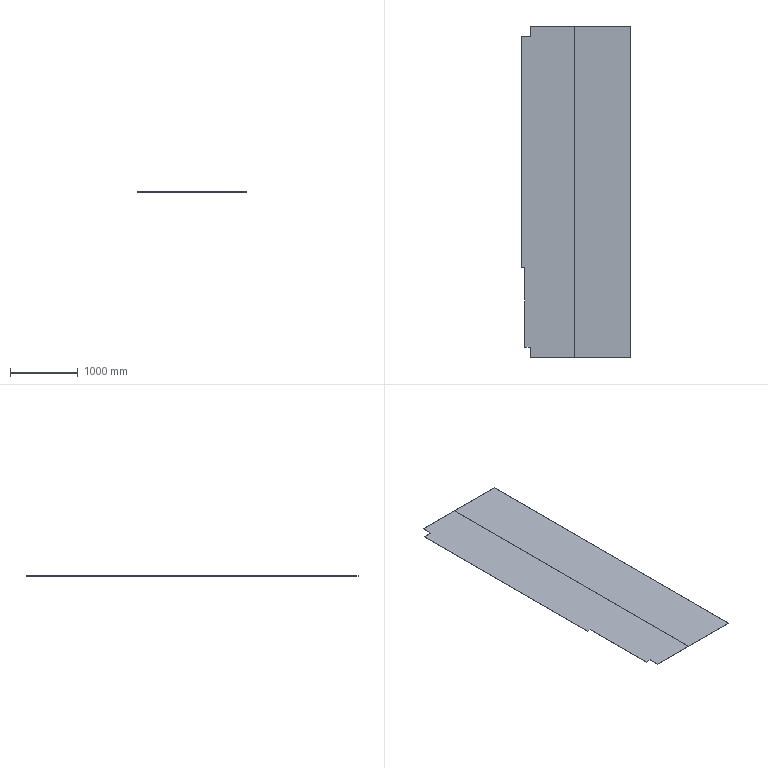Part | STEP file | 休息台花纹Plate 2 | 2 solids | 18 faces | box 1620 x 4900 x 3 mm | volume 23500005 mm3 | plane 18
STEP:
#1=CARTESIAN_POINT('',(0.,0.,0.));
#2=DIRECTION('',(0.,0.,1.));
#3=DIRECTION('',(1.,0.,0.));
#4=AXIS2_PLACEMENT_3D('',#1,#2,#3);
#5=CARTESIAN_POINT('',(-565.,50.,3.));
#6=VERTEX_POINT('',#5);
#7=CARTESIAN_POINT('',(-565.,50.,0.));
#8=VERTEX_POINT('',#7);
#9=CARTESIAN_POINT('',(-565.,50.,3.));
#10=DIRECTION('',(0.,0.,-1.));
#11=VECTOR('',#10,1.);
#12=LINE('',#9,#11);
#13=CARTESIAN_POINT('',(-565.,50.,-0.01));
#14=DIRECTION('',(-1.,0.,0.));
#15=DIRECTION('',(0.,-1.,0.));
#16=AXIS2_PLACEMENT_3D('',#13,#14,#15);
#17=PLANE('',#16);
#18=CARTESIAN_POINT('',(0.,3.01));
#19=DIRECTION('',(0.,-1.));
#20=VECTOR('',#19,1.);
#21=LINE('',#18,#20);
#22=(GEOMETRIC_REPRESENTATION_CONTEXT(2)PARAMETRIC_REPRESENTATION_CONTEXT()REPRESENTATION_CONTEXT('',''));
#23=DEFINITIONAL_REPRESENTATION('',(#21),#22);
#24=PCURVE('',#17,#23);
#25=CARTESIAN_POINT('',(270.,50.,3.));
#26=DIRECTION('',(0.,-1.,0.));
#27=DIRECTION('',(0.,0.,-1.));
#28=AXIS2_PLACEMENT_3D('',#25,#26,#27);
#29=PLANE('',#28);
#30=CARTESIAN_POINT('',(0.,-835.));
#31=DIRECTION('',(1.,0.));
#32=VECTOR('',#31,1.);
#33=LINE('',#30,#32);
#34=(GEOMETRIC_REPRESENTATION_CONTEXT(2)PARAMETRIC_REPRESENTATION_CONTEXT()REPRESENTATION_CONTEXT('',''));
#35=DEFINITIONAL_REPRESENTATION('',(#33),#34);
#36=PCURVE('',#29,#35);
#37=SURFACE_CURVE('',#12,(#24,#36),.PCURVE_S1.);
#38=EDGE_CURVE('',#6,#8,#37,.T.);
#39=ORIENTED_EDGE('',*,*,#38,.F.);
#40=CARTESIAN_POINT('',(-565.,-4850.,3.));
#41=VERTEX_POINT('',#40);
#42=CARTESIAN_POINT('',(-565.,0.,3.));
#43=DIRECTION('',(0.,-1.,0.));
#44=VECTOR('',#43,1.);
#45=LINE('',#42,#44);
#46=CARTESIAN_POINT('',(50.,3.01));
#47=DIRECTION('',(1.,0.));
#48=VECTOR('',#47,1.);
#49=LINE('',#46,#48);
#50=(GEOMETRIC_REPRESENTATION_CONTEXT(2)PARAMETRIC_REPRESENTATION_CONTEXT()REPRESENTATION_CONTEXT('',''));
#51=DEFINITIONAL_REPRESENTATION('',(#49),#50);
#52=PCURVE('',#17,#51);
#53=CARTESIAN_POINT('',(0.,0.,3.));
#54=DIRECTION('',(0.,0.,1.));
#55=DIRECTION('',(1.,0.,0.));
#56=AXIS2_PLACEMENT_3D('',#53,#54,#55);
#57=PLANE('',#56);
#58=CARTESIAN_POINT('',(-565.,0.));
#59=DIRECTION('',(0.,-1.));
#60=VECTOR('',#59,1.);
#61=LINE('',#58,#60);
#62=(GEOMETRIC_REPRESENTATION_CONTEXT(2)PARAMETRIC_REPRESENTATION_CONTEXT()REPRESENTATION_CONTEXT('',''));
#63=DEFINITIONAL_REPRESENTATION('',(#61),#62);
#64=PCURVE('',#57,#63);
#65=SURFACE_CURVE('',#45,(#52,#64),.PCURVE_S1.);
#66=EDGE_CURVE('',#6,#41,#65,.T.);
#67=ORIENTED_EDGE('',*,*,#66,.T.);
#68=CARTESIAN_POINT('',(-565.,-4850.,0.));
#69=VERTEX_POINT('',#68);
#70=CARTESIAN_POINT('',(-565.,-4850.,3.));
#71=DIRECTION('',(0.,0.,1.));
#72=VECTOR('',#71,1.);
#73=LINE('',#70,#72);
#74=CARTESIAN_POINT('',(4900.,3.01));
#75=DIRECTION('',(0.,1.));
#76=VECTOR('',#75,1.);
#77=LINE('',#74,#76);
#78=(GEOMETRIC_REPRESENTATION_CONTEXT(2)PARAMETRIC_REPRESENTATION_CONTEXT()REPRESENTATION_CONTEXT('',''));
#79=DEFINITIONAL_REPRESENTATION('',(#77),#78);
#80=PCURVE('',#17,#79);
#81=CARTESIAN_POINT('',(-1215.,-4850.,3.));
#82=DIRECTION('',(0.,1.,0.));
#83=DIRECTION('',(0.,0.,1.));
#84=AXIS2_PLACEMENT_3D('',#81,#82,#83);
#85=PLANE('',#84);
#86=CARTESIAN_POINT('',(0.,650.));
#87=DIRECTION('',(1.,0.));
#88=VECTOR('',#87,1.);
#89=LINE('',#86,#88);
#90=(GEOMETRIC_REPRESENTATION_CONTEXT(2)PARAMETRIC_REPRESENTATION_CONTEXT()REPRESENTATION_CONTEXT('',''));
#91=DEFINITIONAL_REPRESENTATION('',(#89),#90);
#92=PCURVE('',#85,#91);
#93=SURFACE_CURVE('',#73,(#80,#92),.PCURVE_S1.);
#94=EDGE_CURVE('',#69,#41,#93,.T.);
#95=ORIENTED_EDGE('',*,*,#94,.F.);
#96=CARTESIAN_POINT('',(-565.,0.,0.));
#97=DIRECTION('',(0.,-1.,0.));
#98=VECTOR('',#97,1.);
#99=LINE('',#96,#98);
#100=CARTESIAN_POINT('',(50.,0.01));
#101=DIRECTION('',(1.,0.));
#102=VECTOR('',#101,1.);
#103=LINE('',#100,#102);
#104=(GEOMETRIC_REPRESENTATION_CONTEXT(2)PARAMETRIC_REPRESENTATION_CONTEXT()REPRESENTATION_CONTEXT('',''));
#105=DEFINITIONAL_REPRESENTATION('',(#103),#104);
#106=PCURVE('',#17,#105);
#107=CARTESIAN_POINT('',(0.,0.,0.));
#108=DIRECTION('',(0.,0.,1.));
#109=DIRECTION('',(1.,0.,0.));
#110=AXIS2_PLACEMENT_3D('',#107,#108,#109);
#111=PLANE('',#110);
#112=CARTESIAN_POINT('',(-565.,0.));
#113=DIRECTION('',(0.,-1.));
#114=VECTOR('',#113,1.);
#115=LINE('',#112,#114);
#116=(GEOMETRIC_REPRESENTATION_CONTEXT(2)PARAMETRIC_REPRESENTATION_CONTEXT()REPRESENTATION_CONTEXT('',''));
#117=DEFINITIONAL_REPRESENTATION('',(#115),#116);
#118=PCURVE('',#111,#117);
#119=SURFACE_CURVE('',#99,(#106,#118),.PCURVE_S1.);
#120=EDGE_CURVE('',#8,#69,#119,.T.);
#121=ORIENTED_EDGE('',*,*,#120,.F.);
#122=EDGE_LOOP('',(#39,#67,#95,#121));
#123=FACE_BOUND('',#122,.T.);
#124=ADVANCED_FACE('',(#123),#17,.F.);
#125=ORIENTED_EDGE('',*,*,#66,.F.);
#126=CARTESIAN_POINT('',(-1215.,50.,3.));
#127=VERTEX_POINT('',#126);
#128=CARTESIAN_POINT('',(270.,50.,3.));
#129=DIRECTION('',(-1.,0.,0.));
#130=VECTOR('',#129,1.);
#131=LINE('',#128,#130);
#132=CARTESIAN_POINT('',(270.,50.));
#133=DIRECTION('',(-1.,0.));
#134=VECTOR('',#133,1.);
#135=LINE('',#132,#134);
#136=(GEOMETRIC_REPRESENTATION_CONTEXT(2)PARAMETRIC_REPRESENTATION_CONTEXT()REPRESENTATION_CONTEXT('',''));
#137=DEFINITIONAL_REPRESENTATION('',(#135),#136);
#138=PCURVE('',#57,#137);
#139=CARTESIAN_POINT('',(0.,0.));
#140=DIRECTION('',(0.,-1.));
#141=VECTOR('',#140,1.);
#142=LINE('',#139,#141);
#143=(GEOMETRIC_REPRESENTATION_CONTEXT(2)PARAMETRIC_REPRESENTATION_CONTEXT()REPRESENTATION_CONTEXT('',''));
#144=DEFINITIONAL_REPRESENTATION('',(#142),#143);
#145=PCURVE('',#29,#144);
#146=SURFACE_CURVE('',#131,(#138,#145),.PCURVE_S1.);
#147=EDGE_CURVE('',#6,#127,#146,.T.);
#148=ORIENTED_EDGE('',*,*,#147,.T.);
#149=CARTESIAN_POINT('',(-1215.,-107.,3.));
#150=VERTEX_POINT('',#149);
#151=CARTESIAN_POINT('',(-1215.,50.,3.));
#152=DIRECTION('',(0.,-1.,0.));
#153=VECTOR('',#152,1.);
#154=LINE('',#151,#153);
#155=CARTESIAN_POINT('',(-1215.,50.));
#156=DIRECTION('',(0.,-1.));
#157=VECTOR('',#156,1.);
#158=LINE('',#155,#157);
#159=(GEOMETRIC_REPRESENTATION_CONTEXT(2)PARAMETRIC_REPRESENTATION_CONTEXT()REPRESENTATION_CONTEXT('',''));
#160=DEFINITIONAL_REPRESENTATION('',(#158),#159);
#161=PCURVE('',#57,#160);
#162=CARTESIAN_POINT('',(-1215.,50.,3.));
#163=DIRECTION('',(1.,0.,0.));
#164=DIRECTION('',(0.,0.,-1.));
#165=AXIS2_PLACEMENT_3D('',#162,#163,#164);
#166=PLANE('',#165);
#167=CARTESIAN_POINT('',(0.,0.));
#168=DIRECTION('',(0.,-1.));
#169=VECTOR('',#168,1.);
#170=LINE('',#167,#169);
#171=(GEOMETRIC_REPRESENTATION_CONTEXT(2)PARAMETRIC_REPRESENTATION_CONTEXT()REPRESENTATION_CONTEXT('',''));
#172=DEFINITIONAL_REPRESENTATION('',(#170),#171);
#173=PCURVE('',#166,#172);
#174=SURFACE_CURVE('',#154,(#161,#173),.PCURVE_S1.);
#175=EDGE_CURVE('',#127,#150,#174,.T.);
#176=ORIENTED_EDGE('',*,*,#175,.T.);
#177=CARTESIAN_POINT('',(-1350.,-107.,3.));
#178=VERTEX_POINT('',#177);
#179=CARTESIAN_POINT('',(-1215.,-107.,3.));
#180=DIRECTION('',(-1.,0.,0.));
#181=VECTOR('',#180,1.);
#182=LINE('',#179,#181);
#183=CARTESIAN_POINT('',(-1215.,-107.));
#184=DIRECTION('',(-1.,0.));
#185=VECTOR('',#184,1.);
#186=LINE('',#183,#185);
#187=(GEOMETRIC_REPRESENTATION_CONTEXT(2)PARAMETRIC_REPRESENTATION_CONTEXT()REPRESENTATION_CONTEXT('',''));
#188=DEFINITIONAL_REPRESENTATION('',(#186),#187);
#189=PCURVE('',#57,#188);
#190=CARTESIAN_POINT('',(-1215.,-107.,3.));
#191=DIRECTION('',(0.,-1.,0.));
#192=DIRECTION('',(0.,0.,-1.));
#193=AXIS2_PLACEMENT_3D('',#190,#191,#192);
#194=PLANE('',#193);
#195=CARTESIAN_POINT('',(0.,0.));
#196=DIRECTION('',(0.,-1.));
#197=VECTOR('',#196,1.);
#198=LINE('',#195,#197);
#199=(GEOMETRIC_REPRESENTATION_CONTEXT(2)PARAMETRIC_REPRESENTATION_CONTEXT()REPRESENTATION_CONTEXT('',''));
#200=DEFINITIONAL_REPRESENTATION('',(#198),#199);
#201=PCURVE('',#194,#200);
#202=SURFACE_CURVE('',#182,(#189,#201),.PCURVE_S1.);
#203=EDGE_CURVE('',#150,#178,#202,.T.);
#204=ORIENTED_EDGE('',*,*,#203,.T.);
#205=CARTESIAN_POINT('',(-1350.,-3518.,3.));
#206=VERTEX_POINT('',#205);
#207=CARTESIAN_POINT('',(-1350.,-107.,3.));
#208=DIRECTION('',(0.,-1.,0.));
#209=VECTOR('',#208,1.);
#210=LINE('',#207,#209);
#211=CARTESIAN_POINT('',(-1350.,-107.));
#212=DIRECTION('',(0.,-1.));
#213=VECTOR('',#212,1.);
#214=LINE('',#211,#213);
#215=(GEOMETRIC_REPRESENTATION_CONTEXT(2)PARAMETRIC_REPRESENTATION_CONTEXT()REPRESENTATION_CONTEXT('',''));
#216=DEFINITIONAL_REPRESENTATION('',(#214),#215);
#217=PCURVE('',#57,#216);
#218=CARTESIAN_POINT('',(-1350.,-107.,3.));
#219=DIRECTION('',(1.,0.,0.));
#220=DIRECTION('',(0.,1.,0.));
#221=AXIS2_PLACEMENT_3D('',#218,#219,#220);
#222=PLANE('',#221);
#223=CARTESIAN_POINT('',(0.,0.));
#224=DIRECTION('',(-1.,0.));
#225=VECTOR('',#224,1.);
#226=LINE('',#223,#225);
#227=(GEOMETRIC_REPRESENTATION_CONTEXT(2)PARAMETRIC_REPRESENTATION_CONTEXT()REPRESENTATION_CONTEXT('',''));
#228=DEFINITIONAL_REPRESENTATION('',(#226),#227);
#229=PCURVE('',#222,#228);
#230=SURFACE_CURVE('',#210,(#217,#229),.PCURVE_S1.);
#231=EDGE_CURVE('',#178,#206,#230,.T.);
#232=ORIENTED_EDGE('',*,*,#231,.T.);
#233=CARTESIAN_POINT('',(-1297.,-3518.,3.));
#234=VERTEX_POINT('',#233);
#235=CARTESIAN_POINT('',(-1350.,-3518.,3.));
#236=DIRECTION('',(1.,0.,0.));
#237=VECTOR('',#236,1.);
#238=LINE('',#235,#237);
#239=CARTESIAN_POINT('',(-1350.,-3518.));
#240=DIRECTION('',(1.,0.));
#241=VECTOR('',#240,1.);
#242=LINE('',#239,#241);
#243=(GEOMETRIC_REPRESENTATION_CONTEXT(2)PARAMETRIC_REPRESENTATION_CONTEXT()REPRESENTATION_CONTEXT('',''));
#244=DEFINITIONAL_REPRESENTATION('',(#242),#243);
#245=PCURVE('',#57,#244);
#246=CARTESIAN_POINT('',(-1350.,-3518.,3.));
#247=DIRECTION('',(0.,1.,0.));
#248=DIRECTION('',(0.,0.,1.));
#249=AXIS2_PLACEMENT_3D('',#246,#247,#248);
#250=PLANE('',#249);
#251=CARTESIAN_POINT('',(0.,0.));
#252=DIRECTION('',(0.,1.));
#253=VECTOR('',#252,1.);
#254=LINE('',#251,#253);
#255=(GEOMETRIC_REPRESENTATION_CONTEXT(2)PARAMETRIC_REPRESENTATION_CONTEXT()REPRESENTATION_CONTEXT('',''));
#256=DEFINITIONAL_REPRESENTATION('',(#254),#255);
#257=PCURVE('',#250,#256);
#258=SURFACE_CURVE('',#238,(#245,#257),.PCURVE_S1.);
#259=EDGE_CURVE('',#206,#234,#258,.T.);
#260=ORIENTED_EDGE('',*,*,#259,.T.);
#261=CARTESIAN_POINT('',(-1297.,-4693.,3.));
#262=VERTEX_POINT('',#261);
#263=CARTESIAN_POINT('',(-1297.,-3518.,3.));
#264=DIRECTION('',(0.,-1.,0.));
#265=VECTOR('',#264,1.);
#266=LINE('',#263,#265);
#267=CARTESIAN_POINT('',(-1297.,-3518.));
#268=DIRECTION('',(0.,-1.));
#269=VECTOR('',#268,1.);
#270=LINE('',#267,#269);
#271=(GEOMETRIC_REPRESENTATION_CONTEXT(2)PARAMETRIC_REPRESENTATION_CONTEXT()REPRESENTATION_CONTEXT('',''));
#272=DEFINITIONAL_REPRESENTATION('',(#270),#271);
#273=PCURVE('',#57,#272);
#274=CARTESIAN_POINT('',(-1297.,-3518.,3.));
#275=DIRECTION('',(1.,0.,0.));
#276=DIRECTION('',(0.,1.,0.));
#277=AXIS2_PLACEMENT_3D('',#274,#275,#276);
#278=PLANE('',#277);
#279=CARTESIAN_POINT('',(0.,0.));
#280=DIRECTION('',(-1.,0.));
#281=VECTOR('',#280,1.);
#282=LINE('',#279,#281);
#283=(GEOMETRIC_REPRESENTATION_CONTEXT(2)PARAMETRIC_REPRESENTATION_CONTEXT()REPRESENTATION_CONTEXT('',''));
#284=DEFINITIONAL_REPRESENTATION('',(#282),#283);
#285=PCURVE('',#278,#284);
#286=SURFACE_CURVE('',#266,(#273,#285),.PCURVE_S1.);
#287=EDGE_CURVE('',#234,#262,#286,.T.);
#288=ORIENTED_EDGE('',*,*,#287,.T.);
#289=CARTESIAN_POINT('',(-1215.,-4693.,3.));
#290=VERTEX_POINT('',#289);
#291=CARTESIAN_POINT('',(-1297.,-4693.,3.));
#292=DIRECTION('',(1.,0.,0.));
#293=VECTOR('',#292,1.);
#294=LINE('',#291,#293);
#295=CARTESIAN_POINT('',(-1297.,-4693.));
#296=DIRECTION('',(1.,0.));
#297=VECTOR('',#296,1.);
#298=LINE('',#295,#297);
#299=(GEOMETRIC_REPRESENTATION_CONTEXT(2)PARAMETRIC_REPRESENTATION_CONTEXT()REPRESENTATION_CONTEXT('',''));
#300=DEFINITIONAL_REPRESENTATION('',(#298),#299);
#301=PCURVE('',#57,#300);
#302=CARTESIAN_POINT('',(-1297.,-4693.,3.));
#303=DIRECTION('',(0.,1.,0.));
#304=DIRECTION('',(0.,0.,1.));
#305=AXIS2_PLACEMENT_3D('',#302,#303,#304);
#306=PLANE('',#305);
#307=CARTESIAN_POINT('',(0.,0.));
#308=DIRECTION('',(0.,1.));
#309=VECTOR('',#308,1.);
#310=LINE('',#307,#309);
#311=(GEOMETRIC_REPRESENTATION_CONTEXT(2)PARAMETRIC_REPRESENTATION_CONTEXT()REPRESENTATION_CONTEXT('',''));
#312=DEFINITIONAL_REPRESENTATION('',(#310),#311);
#313=PCURVE('',#306,#312);
#314=SURFACE_CURVE('',#294,(#301,#313),.PCURVE_S1.);
#315=EDGE_CURVE('',#262,#290,#314,.T.);
#316=ORIENTED_EDGE('',*,*,#315,.T.);
#317=CARTESIAN_POINT('',(-1215.,-4850.,3.));
#318=VERTEX_POINT('',#317);
#319=CARTESIAN_POINT('',(-1215.,-4693.,3.));
#320=DIRECTION('',(0.,-1.,0.));
#321=VECTOR('',#320,1.);
#322=LINE('',#319,#321);
#323=CARTESIAN_POINT('',(-1215.,-4693.));
#324=DIRECTION('',(0.,-1.));
#325=VECTOR('',#324,1.);
#326=LINE('',#323,#325);
#327=(GEOMETRIC_REPRESENTATION_CONTEXT(2)PARAMETRIC_REPRESENTATION_CONTEXT()REPRESENTATION_CONTEXT('',''));
#328=DEFINITIONAL_REPRESENTATION('',(#326),#327);
#329=PCURVE('',#57,#328);
#330=CARTESIAN_POINT('',(-1215.,-4693.,3.));
#331=DIRECTION('',(1.,0.,0.));
#332=DIRECTION('',(0.,0.,-1.));
#333=AXIS2_PLACEMENT_3D('',#330,#331,#332);
#334=PLANE('',#333);
#335=CARTESIAN_POINT('',(0.,0.));
#336=DIRECTION('',(0.,-1.));
#337=VECTOR('',#336,1.);
#338=LINE('',#335,#337);
#339=(GEOMETRIC_REPRESENTATION_CONTEXT(2)PARAMETRIC_REPRESENTATION_CONTEXT()REPRESENTATION_CONTEXT('',''));
#340=DEFINITIONAL_REPRESENTATION('',(#338),#339);
#341=PCURVE('',#334,#340);
#342=SURFACE_CURVE('',#322,(#329,#341),.PCURVE_S1.);
#343=EDGE_CURVE('',#290,#318,#342,.T.);
#344=ORIENTED_EDGE('',*,*,#343,.T.);
#345=CARTESIAN_POINT('',(-1215.,-4850.,3.));
#346=DIRECTION('',(1.,0.,0.));
#347=VECTOR('',#346,1.);
#348=LINE('',#345,#347);
#349=CARTESIAN_POINT('',(-1215.,-4850.));
#350=DIRECTION('',(1.,0.));
#351=VECTOR('',#350,1.);
#352=LINE('',#349,#351);
#353=(GEOMETRIC_REPRESENTATION_CONTEXT(2)PARAMETRIC_REPRESENTATION_CONTEXT()REPRESENTATION_CONTEXT('',''));
#354=DEFINITIONAL_REPRESENTATION('',(#352),#353);
#355=PCURVE('',#57,#354);
#356=CARTESIAN_POINT('',(0.,0.));
#357=DIRECTION('',(0.,1.));
#358=VECTOR('',#357,1.);
#359=LINE('',#356,#358);
#360=(GEOMETRIC_REPRESENTATION_CONTEXT(2)PARAMETRIC_REPRESENTATION_CONTEXT()REPRESENTATION_CONTEXT('',''));
#361=DEFINITIONAL_REPRESENTATION('',(#359),#360);
#362=PCURVE('',#85,#361);
#363=SURFACE_CURVE('',#348,(#355,#362),.PCURVE_S1.);
#364=EDGE_CURVE('',#318,#41,#363,.T.);
#365=ORIENTED_EDGE('',*,*,#364,.T.);
#366=EDGE_LOOP('',(#125,#148,#176,#204,#232,#260,#288,#316,#344,#365));
#367=FACE_BOUND('',#366,.T.);
#368=ADVANCED_FACE('',(#367),#57,.T.);
#369=CARTESIAN_POINT('',(-1215.,50.,0.));
#370=VERTEX_POINT('',#369);
#371=CARTESIAN_POINT('',(270.,50.,0.));
#372=DIRECTION('',(-1.,0.,0.));
#373=VECTOR('',#372,1.);
#374=LINE('',#371,#373);
#375=CARTESIAN_POINT('',(270.,50.));
#376=DIRECTION('',(-1.,0.));
#377=VECTOR('',#376,1.);
#378=LINE('',#375,#377);
#379=(GEOMETRIC_REPRESENTATION_CONTEXT(2)PARAMETRIC_REPRESENTATION_CONTEXT()REPRESENTATION_CONTEXT('',''));
#380=DEFINITIONAL_REPRESENTATION('',(#378),#379);
#381=PCURVE('',#111,#380);
#382=CARTESIAN_POINT('',(3.,0.));
#383=DIRECTION('',(0.,-1.));
#384=VECTOR('',#383,1.);
#385=LINE('',#382,#384);
#386=(GEOMETRIC_REPRESENTATION_CONTEXT(2)PARAMETRIC_REPRESENTATION_CONTEXT()REPRESENTATION_CONTEXT('',''));
#387=DEFINITIONAL_REPRESENTATION('',(#385),#386);
#388=PCURVE('',#29,#387);
#389=SURFACE_CURVE('',#374,(#381,#388),.PCURVE_S1.);
#390=EDGE_CURVE('',#8,#370,#389,.T.);
#391=ORIENTED_EDGE('',*,*,#390,.F.);
#392=ORIENTED_EDGE('',*,*,#120,.T.);
#393=CARTESIAN_POINT('',(-1215.,-4850.,0.));
#394=VERTEX_POINT('',#393);
#395=CARTESIAN_POINT('',(-1215.,-4850.,0.));
#396=DIRECTION('',(1.,0.,0.));
#397=VECTOR('',#396,1.);
#398=LINE('',#395,#397);
#399=CARTESIAN_POINT('',(-1215.,-4850.));
#400=DIRECTION('',(1.,0.));
#401=VECTOR('',#400,1.);
#402=LINE('',#399,#401);
#403=(GEOMETRIC_REPRESENTATION_CONTEXT(2)PARAMETRIC_REPRESENTATION_CONTEXT()REPRESENTATION_CONTEXT('',''));
#404=DEFINITIONAL_REPRESENTATION('',(#402),#403);
#405=PCURVE('',#111,#404);
#406=CARTESIAN_POINT('',(-3.,0.));
#407=DIRECTION('',(0.,1.));
#408=VECTOR('',#407,1.);
#409=LINE('',#406,#408);
#410=(GEOMETRIC_REPRESENTATION_CONTEXT(2)PARAMETRIC_REPRESENTATION_CONTEXT()REPRESENTATION_CONTEXT('',''));
#411=DEFINITIONAL_REPRESENTATION('',(#409),#410);
#412=PCURVE('',#85,#411);
#413=SURFACE_CURVE('',#398,(#405,#412),.PCURVE_S1.);
#414=EDGE_CURVE('',#394,#69,#413,.T.);
#415=ORIENTED_EDGE('',*,*,#414,.F.);
#416=CARTESIAN_POINT('',(-1215.,-4693.,0.));
#417=VERTEX_POINT('',#416);
#418=CARTESIAN_POINT('',(-1215.,-4693.,0.));
#419=DIRECTION('',(0.,-1.,0.));
#420=VECTOR('',#419,1.);
#421=LINE('',#418,#420);
#422=CARTESIAN_POINT('',(-1215.,-4693.));
#423=DIRECTION('',(0.,-1.));
#424=VECTOR('',#423,1.);
#425=LINE('',#422,#424);
#426=(GEOMETRIC_REPRESENTATION_CONTEXT(2)PARAMETRIC_REPRESENTATION_CONTEXT()REPRESENTATION_CONTEXT('',''));
#427=DEFINITIONAL_REPRESENTATION('',(#425),#426);
#428=PCURVE('',#111,#427);
#429=CARTESIAN_POINT('',(3.,0.));
#430=DIRECTION('',(0.,-1.));
#431=VECTOR('',#430,1.);
#432=LINE('',#429,#431);
#433=(GEOMETRIC_REPRESENTATION_CONTEXT(2)PARAMETRIC_REPRESENTATION_CONTEXT()REPRESENTATION_CONTEXT('',''));
#434=DEFINITIONAL_REPRESENTATION('',(#432),#433);
#435=PCURVE('',#334,#434);
#436=SURFACE_CURVE('',#421,(#428,#435),.PCURVE_S1.);
#437=EDGE_CURVE('',#417,#394,#436,.T.);
#438=ORIENTED_EDGE('',*,*,#437,.F.);
#439=CARTESIAN_POINT('',(-1297.,-4693.,0.));
#440=VERTEX_POINT('',#439);
#441=CARTESIAN_POINT('',(-1297.,-4693.,0.));
#442=DIRECTION('',(1.,0.,0.));
#443=VECTOR('',#442,1.);
#444=LINE('',#441,#443);
#445=CARTESIAN_POINT('',(-1297.,-4693.));
#446=DIRECTION('',(1.,0.));
#447=VECTOR('',#446,1.);
#448=LINE('',#445,#447);
#449=(GEOMETRIC_REPRESENTATION_CONTEXT(2)PARAMETRIC_REPRESENTATION_CONTEXT()REPRESENTATION_CONTEXT('',''));
#450=DEFINITIONAL_REPRESENTATION('',(#448),#449);
#451=PCURVE('',#111,#450);
#452=CARTESIAN_POINT('',(-3.,0.));
#453=DIRECTION('',(0.,1.));
#454=VECTOR('',#453,1.);
#455=LINE('',#452,#454);
#456=(GEOMETRIC_REPRESENTATION_CONTEXT(2)PARAMETRIC_REPRESENTATION_CONTEXT()REPRESENTATION_CONTEXT('',''));
#457=DEFINITIONAL_REPRESENTATION('',(#455),#456);
#458=PCURVE('',#306,#457);
#459=SURFACE_CURVE('',#444,(#451,#458),.PCURVE_S1.);
#460=EDGE_CURVE('',#440,#417,#459,.T.);
#461=ORIENTED_EDGE('',*,*,#460,.F.);
#462=CARTESIAN_POINT('',(-1297.,-3518.,0.));
#463=VERTEX_POINT('',#462);
#464=CARTESIAN_POINT('',(-1297.,-3518.,0.));
#465=DIRECTION('',(0.,-1.,0.));
#466=VECTOR('',#465,1.);
#467=LINE('',#464,#466);
#468=CARTESIAN_POINT('',(-1297.,-3518.));
#469=DIRECTION('',(0.,-1.));
#470=VECTOR('',#469,1.);
#471=LINE('',#468,#470);
#472=(GEOMETRIC_REPRESENTATION_CONTEXT(2)PARAMETRIC_REPRESENTATION_CONTEXT()REPRESENTATION_CONTEXT('',''));
#473=DEFINITIONAL_REPRESENTATION('',(#471),#472);
#474=PCURVE('',#111,#473);
#475=CARTESIAN_POINT('',(0.,-3.));
#476=DIRECTION('',(-1.,0.));
#477=VECTOR('',#476,1.);
#478=LINE('',#475,#477);
#479=(GEOMETRIC_REPRESENTATION_CONTEXT(2)PARAMETRIC_REPRESENTATION_CONTEXT()REPRESENTATION_CONTEXT('',''));
#480=DEFINITIONAL_REPRESENTATION('',(#478),#479);
#481=PCURVE('',#278,#480);
#482=SURFACE_CURVE('',#467,(#474,#481),.PCURVE_S1.);
#483=EDGE_CURVE('',#463,#440,#482,.T.);
#484=ORIENTED_EDGE('',*,*,#483,.F.);
#485=CARTESIAN_POINT('',(-1350.,-3518.,0.));
#486=VERTEX_POINT('',#485);
#487=CARTESIAN_POINT('',(-1350.,-3518.,0.));
#488=DIRECTION('',(1.,0.,0.));
#489=VECTOR('',#488,1.);
#490=LINE('',#487,#489);
#491=CARTESIAN_POINT('',(-1350.,-3518.));
#492=DIRECTION('',(1.,0.));
#493=VECTOR('',#492,1.);
#494=LINE('',#491,#493);
#495=(GEOMETRIC_REPRESENTATION_CONTEXT(2)PARAMETRIC_REPRESENTATION_CONTEXT()REPRESENTATION_CONTEXT('',''));
#496=DEFINITIONAL_REPRESENTATION('',(#494),#495);
#497=PCURVE('',#111,#496);
#498=CARTESIAN_POINT('',(-3.,0.));
#499=DIRECTION('',(0.,1.));
#500=VECTOR('',#499,1.);
#501=LINE('',#498,#500);
#502=(GEOMETRIC_REPRESENTATION_CONTEXT(2)PARAMETRIC_REPRESENTATION_CONTEXT()REPRESENTATION_CONTEXT('',''));
#503=DEFINITIONAL_REPRESENTATION('',(#501),#502);
#504=PCURVE('',#250,#503);
#505=SURFACE_CURVE('',#490,(#497,#504),.PCURVE_S1.);
#506=EDGE_CURVE('',#486,#463,#505,.T.);
#507=ORIENTED_EDGE('',*,*,#506,.F.);
#508=CARTESIAN_POINT('',(-1350.,-107.,0.));
#509=VERTEX_POINT('',#508);
#510=CARTESIAN_POINT('',(-1350.,-107.,0.));
#511=DIRECTION('',(0.,-1.,0.));
#512=VECTOR('',#511,1.);
#513=LINE('',#510,#512);
#514=CARTESIAN_POINT('',(-1350.,-107.));
#515=DIRECTION('',(0.,-1.));
#516=VECTOR('',#515,1.);
#517=LINE('',#514,#516);
#518=(GEOMETRIC_REPRESENTATION_CONTEXT(2)PARAMETRIC_REPRESENTATION_CONTEXT()REPRESENTATION_CONTEXT('',''));
#519=DEFINITIONAL_REPRESENTATION('',(#517),#518);
#520=PCURVE('',#111,#519);
#521=CARTESIAN_POINT('',(0.,-3.));
#522=DIRECTION('',(-1.,0.));
#523=VECTOR('',#522,1.);
#524=LINE('',#521,#523);
#525=(GEOMETRIC_REPRESENTATION_CONTEXT(2)PARAMETRIC_REPRESENTATION_CONTEXT()REPRESENTATION_CONTEXT('',''));
#526=DEFINITIONAL_REPRESENTATION('',(#524),#525);
#527=PCURVE('',#222,#526);
#528=SURFACE_CURVE('',#513,(#520,#527),.PCURVE_S1.);
#529=EDGE_CURVE('',#509,#486,#528,.T.);
#530=ORIENTED_EDGE('',*,*,#529,.F.);
#531=CARTESIAN_POINT('',(-1215.,-107.,0.));
#532=VERTEX_POINT('',#531);
#533=CARTESIAN_POINT('',(-1215.,-107.,0.));
#534=DIRECTION('',(-1.,0.,0.));
#535=VECTOR('',#534,1.);
#536=LINE('',#533,#535);
#537=CARTESIAN_POINT('',(-1215.,-107.));
#538=DIRECTION('',(-1.,0.));
#539=VECTOR('',#538,1.);
#540=LINE('',#537,#539);
#541=(GEOMETRIC_REPRESENTATION_CONTEXT(2)PARAMETRIC_REPRESENTATION_CONTEXT()REPRESENTATION_CONTEXT('',''));
#542=DEFINITIONAL_REPRESENTATION('',(#540),#541);
#543=PCURVE('',#111,#542);
#544=CARTESIAN_POINT('',(3.,0.));
#545=DIRECTION('',(0.,-1.));
#546=VECTOR('',#545,1.);
#547=LINE('',#544,#546);
#548=(GEOMETRIC_REPRESENTATION_CONTEXT(2)PARAMETRIC_REPRESENTATION_CONTEXT()REPRESENTATION_CONTEXT('',''));
#549=DEFINITIONAL_REPRESENTATION('',(#547),#548);
#550=PCURVE('',#194,#549);
#551=SURFACE_CURVE('',#536,(#543,#550),.PCURVE_S1.);
#552=EDGE_CURVE('',#532,#509,#551,.T.);
#553=ORIENTED_EDGE('',*,*,#552,.F.);
#554=CARTESIAN_POINT('',(-1215.,50.,0.));
#555=DIRECTION('',(0.,-1.,0.));
#556=VECTOR('',#555,1.);
#557=LINE('',#554,#556);
#558=CARTESIAN_POINT('',(-1215.,50.));
#559=DIRECTION('',(0.,-1.));
#560=VECTOR('',#559,1.);
#561=LINE('',#558,#560);
#562=(GEOMETRIC_REPRESENTATION_CONTEXT(2)PARAMETRIC_REPRESENTATION_CONTEXT()REPRESENTATION_CONTEXT('',''));
#563=DEFINITIONAL_REPRESENTATION('',(#561),#562);
#564=PCURVE('',#111,#563);
#565=CARTESIAN_POINT('',(3.,0.));
#566=DIRECTION('',(0.,-1.));
#567=VECTOR('',#566,1.);
#568=LINE('',#565,#567);
#569=(GEOMETRIC_REPRESENTATION_CONTEXT(2)PARAMETRIC_REPRESENTATION_CONTEXT()REPRESENTATION_CONTEXT('',''));
#570=DEFINITIONAL_REPRESENTATION('',(#568),#569);
#571=PCURVE('',#166,#570);
#572=SURFACE_CURVE('',#557,(#564,#571),.PCURVE_S1.);
#573=EDGE_CURVE('',#370,#532,#572,.T.);
#574=ORIENTED_EDGE('',*,*,#573,.F.);
#575=EDGE_LOOP('',(#391,#392,#415,#438,#461,#484,#507,#530,#553,#574));
#576=FACE_BOUND('',#575,.T.);
#577=ADVANCED_FACE('',(#576),#111,.F.);
#578=ORIENTED_EDGE('',*,*,#147,.F.);
#579=ORIENTED_EDGE('',*,*,#38,.T.);
#580=ORIENTED_EDGE('',*,*,#390,.T.);
#581=CARTESIAN_POINT('',(-1215.,50.,3.));
#582=DIRECTION('',(0.,0.,-1.));
#583=VECTOR('',#582,1.);
#584=LINE('',#581,#583);
#585=CARTESIAN_POINT('',(0.,-1485.));
#586=DIRECTION('',(1.,0.));
#587=VECTOR('',#586,1.);
#588=LINE('',#585,#587);
#589=(GEOMETRIC_REPRESENTATION_CONTEXT(2)PARAMETRIC_REPRESENTATION_CONTEXT()REPRESENTATION_CONTEXT('',''));
#590=DEFINITIONAL_REPRESENTATION('',(#588),#589);
#591=PCURVE('',#29,#590);
#592=CARTESIAN_POINT('',(0.,0.));
#593=DIRECTION('',(1.,0.));
#594=VECTOR('',#593,1.);
#595=LINE('',#592,#594);
#596=(GEOMETRIC_REPRESENTATION_CONTEXT(2)PARAMETRIC_REPRESENTATION_CONTEXT()REPRESENTATION_CONTEXT('',''));
#597=DEFINITIONAL_REPRESENTATION('',(#595),#596);
#598=PCURVE('',#166,#597);
#599=SURFACE_CURVE('',#584,(#591,#598),.PCURVE_S1.);
#600=EDGE_CURVE('',#127,#370,#599,.T.);
#601=ORIENTED_EDGE('',*,*,#600,.F.);
#602=EDGE_LOOP('',(#578,#579,#580,#601));
#603=FACE_BOUND('',#602,.T.);
#604=ADVANCED_FACE('',(#603),#29,.F.);
#605=ORIENTED_EDGE('',*,*,#414,.T.);
#606=ORIENTED_EDGE('',*,*,#94,.T.);
#607=ORIENTED_EDGE('',*,*,#364,.F.);
#608=CARTESIAN_POINT('',(-1215.,-4850.,3.));
#609=DIRECTION('',(0.,0.,-1.));
#610=VECTOR('',#609,1.);
#611=LINE('',#608,#610);
#612=CARTESIAN_POINT('',(0.,0.));
#613=DIRECTION('',(-1.,0.));
#614=VECTOR('',#613,1.);
#615=LINE('',#612,#614);
#616=(GEOMETRIC_REPRESENTATION_CONTEXT(2)PARAMETRIC_REPRESENTATION_CONTEXT()REPRESENTATION_CONTEXT('',''));
#617=DEFINITIONAL_REPRESENTATION('',(#615),#616);
#618=PCURVE('',#85,#617);
#619=CARTESIAN_POINT('',(0.,-157.));
#620=DIRECTION('',(1.,0.));
#621=VECTOR('',#620,1.);
#622=LINE('',#619,#621);
#623=(GEOMETRIC_REPRESENTATION_CONTEXT(2)PARAMETRIC_REPRESENTATION_CONTEXT()REPRESENTATION_CONTEXT('',''));
#624=DEFINITIONAL_REPRESENTATION('',(#622),#623);
#625=PCURVE('',#334,#624);
#626=SURFACE_CURVE('',#611,(#618,#625),.PCURVE_S1.);
#627=EDGE_CURVE('',#318,#394,#626,.T.);
#628=ORIENTED_EDGE('',*,*,#627,.T.);
#629=EDGE_LOOP('',(#605,#606,#607,#628));
#630=FACE_BOUND('',#629,.T.);
#631=ADVANCED_FACE('',(#630),#85,.F.);
#632=ORIENTED_EDGE('',*,*,#437,.T.);
#633=ORIENTED_EDGE('',*,*,#627,.F.);
#634=ORIENTED_EDGE('',*,*,#343,.F.);
#635=CARTESIAN_POINT('',(-1215.,-4693.,3.));
#636=DIRECTION('',(0.,0.,-1.));
#637=VECTOR('',#636,1.);
#638=LINE('',#635,#637);
#639=CARTESIAN_POINT('',(0.,0.));
#640=DIRECTION('',(1.,0.));
#641=VECTOR('',#640,1.);
#642=LINE('',#639,#641);
#643=(GEOMETRIC_REPRESENTATION_CONTEXT(2)PARAMETRIC_REPRESENTATION_CONTEXT()REPRESENTATION_CONTEXT('',''));
#644=DEFINITIONAL_REPRESENTATION('',(#642),#643);
#645=PCURVE('',#334,#644);
#646=CARTESIAN_POINT('',(0.,82.));
#647=DIRECTION('',(-1.,0.));
#648=VECTOR('',#647,1.);
#649=LINE('',#646,#648);
#650=(GEOMETRIC_REPRESENTATION_CONTEXT(2)PARAMETRIC_REPRESENTATION_CONTEXT()REPRESENTATION_CONTEXT('',''));
#651=DEFINITIONAL_REPRESENTATION('',(#649),#650);
#652=PCURVE('',#306,#651);
#653=SURFACE_CURVE('',#638,(#645,#652),.PCURVE_S1.);
#654=EDGE_CURVE('',#290,#417,#653,.T.);
#655=ORIENTED_EDGE('',*,*,#654,.T.);
#656=EDGE_LOOP('',(#632,#633,#634,#655));
#657=FACE_BOUND('',#656,.T.);
#658=ADVANCED_FACE('',(#657),#334,.F.);
#659=ORIENTED_EDGE('',*,*,#460,.T.);
#660=ORIENTED_EDGE('',*,*,#654,.F.);
#661=ORIENTED_EDGE('',*,*,#315,.F.);
#662=CARTESIAN_POINT('',(-1297.,-4693.,3.));
#663=DIRECTION('',(0.,0.,-1.));
#664=VECTOR('',#663,1.);
#665=LINE('',#662,#664);
#666=CARTESIAN_POINT('',(0.,0.));
#667=DIRECTION('',(-1.,0.));
#668=VECTOR('',#667,1.);
#669=LINE('',#666,#668);
#670=(GEOMETRIC_REPRESENTATION_CONTEXT(2)PARAMETRIC_REPRESENTATION_CONTEXT()REPRESENTATION_CONTEXT('',''));
#671=DEFINITIONAL_REPRESENTATION('',(#669),#670);
#672=PCURVE('',#306,#671);
#673=CARTESIAN_POINT('',(-1175.,0.));
#674=DIRECTION('',(0.,-1.));
#675=VECTOR('',#674,1.);
#676=LINE('',#673,#675);
#677=(GEOMETRIC_REPRESENTATION_CONTEXT(2)PARAMETRIC_REPRESENTATION_CONTEXT()REPRESENTATION_CONTEXT('',''));
#678=DEFINITIONAL_REPRESENTATION('',(#676),#677);
#679=PCURVE('',#278,#678);
#680=SURFACE_CURVE('',#665,(#672,#679),.PCURVE_S1.);
#681=EDGE_CURVE('',#262,#440,#680,.T.);
#682=ORIENTED_EDGE('',*,*,#681,.T.);
#683=EDGE_LOOP('',(#659,#660,#661,#682));
#684=FACE_BOUND('',#683,.T.);
#685=ADVANCED_FACE('',(#684),#306,.F.);
#686=ORIENTED_EDGE('',*,*,#483,.T.);
#687=ORIENTED_EDGE('',*,*,#681,.F.);
#688=ORIENTED_EDGE('',*,*,#287,.F.);
#689=CARTESIAN_POINT('',(-1297.,-3518.,3.));
#690=DIRECTION('',(0.,0.,-1.));
#691=VECTOR('',#690,1.);
#692=LINE('',#689,#691);
#693=CARTESIAN_POINT('',(0.,0.));
#694=DIRECTION('',(0.,-1.));
#695=VECTOR('',#694,1.);
#696=LINE('',#693,#695);
#697=(GEOMETRIC_REPRESENTATION_CONTEXT(2)PARAMETRIC_REPRESENTATION_CONTEXT()REPRESENTATION_CONTEXT('',''));
#698=DEFINITIONAL_REPRESENTATION('',(#696),#697);
#699=PCURVE('',#278,#698);
#700=CARTESIAN_POINT('',(0.,53.));
#701=DIRECTION('',(-1.,0.));
#702=VECTOR('',#701,1.);
#703=LINE('',#700,#702);
#704=(GEOMETRIC_REPRESENTATION_CONTEXT(2)PARAMETRIC_REPRESENTATION_CONTEXT()REPRESENTATION_CONTEXT('',''));
#705=DEFINITIONAL_REPRESENTATION('',(#703),#704);
#706=PCURVE('',#250,#705);
#707=SURFACE_CURVE('',#692,(#699,#706),.PCURVE_S1.);
#708=EDGE_CURVE('',#234,#463,#707,.T.);
#709=ORIENTED_EDGE('',*,*,#708,.T.);
#710=EDGE_LOOP('',(#686,#687,#688,#709));
#711=FACE_BOUND('',#710,.T.);
#712=ADVANCED_FACE('',(#711),#278,.F.);
#713=ORIENTED_EDGE('',*,*,#506,.T.);
#714=ORIENTED_EDGE('',*,*,#708,.F.);
#715=ORIENTED_EDGE('',*,*,#259,.F.);
#716=CARTESIAN_POINT('',(-1350.,-3518.,3.));
#717=DIRECTION('',(0.,0.,-1.));
#718=VECTOR('',#717,1.);
#719=LINE('',#716,#718);
#720=CARTESIAN_POINT('',(0.,0.));
#721=DIRECTION('',(-1.,0.));
#722=VECTOR('',#721,1.);
#723=LINE('',#720,#722);
#724=(GEOMETRIC_REPRESENTATION_CONTEXT(2)PARAMETRIC_REPRESENTATION_CONTEXT()REPRESENTATION_CONTEXT('',''));
#725=DEFINITIONAL_REPRESENTATION('',(#723),#724);
#726=PCURVE('',#250,#725);
#727=CARTESIAN_POINT('',(-3411.,0.));
#728=DIRECTION('',(0.,-1.));
#729=VECTOR('',#728,1.);
#730=LINE('',#727,#729);
#731=(GEOMETRIC_REPRESENTATION_CONTEXT(2)PARAMETRIC_REPRESENTATION_CONTEXT()REPRESENTATION_CONTEXT('',''));
#732=DEFINITIONAL_REPRESENTATION('',(#730),#731);
#733=PCURVE('',#222,#732);
#734=SURFACE_CURVE('',#719,(#726,#733),.PCURVE_S1.);
#735=EDGE_CURVE('',#206,#486,#734,.T.);
#736=ORIENTED_EDGE('',*,*,#735,.T.);
#737=EDGE_LOOP('',(#713,#714,#715,#736));
#738=FACE_BOUND('',#737,.T.);
#739=ADVANCED_FACE('',(#738),#250,.F.);
#740=ORIENTED_EDGE('',*,*,#529,.T.);
#741=ORIENTED_EDGE('',*,*,#735,.F.);
#742=ORIENTED_EDGE('',*,*,#231,.F.);
#743=CARTESIAN_POINT('',(-1350.,-107.,3.));
#744=DIRECTION('',(0.,0.,-1.));
#745=VECTOR('',#744,1.);
#746=LINE('',#743,#745);
#747=CARTESIAN_POINT('',(0.,0.));
#748=DIRECTION('',(0.,-1.));
#749=VECTOR('',#748,1.);
#750=LINE('',#747,#749);
#751=(GEOMETRIC_REPRESENTATION_CONTEXT(2)PARAMETRIC_REPRESENTATION_CONTEXT()REPRESENTATION_CONTEXT('',''));
#752=DEFINITIONAL_REPRESENTATION('',(#750),#751);
#753=PCURVE('',#222,#752);
#754=CARTESIAN_POINT('',(0.,-135.));
#755=DIRECTION('',(1.,0.));
#756=VECTOR('',#755,1.);
#757=LINE('',#754,#756);
#758=(GEOMETRIC_REPRESENTATION_CONTEXT(2)PARAMETRIC_REPRESENTATION_CONTEXT()REPRESENTATION_CONTEXT('',''));
#759=DEFINITIONAL_REPRESENTATION('',(#757),#758);
#760=PCURVE('',#194,#759);
#761=SURFACE_CURVE('',#746,(#753,#760),.PCURVE_S1.);
#762=EDGE_CURVE('',#178,#509,#761,.T.);
#763=ORIENTED_EDGE('',*,*,#762,.T.);
#764=EDGE_LOOP('',(#740,#741,#742,#763));
#765=FACE_BOUND('',#764,.T.);
#766=ADVANCED_FACE('',(#765),#222,.F.);
#767=ORIENTED_EDGE('',*,*,#552,.T.);
#768=ORIENTED_EDGE('',*,*,#762,.F.);
#769=ORIENTED_EDGE('',*,*,#203,.F.);
#770=CARTESIAN_POINT('',(-1215.,-107.,3.));
#771=DIRECTION('',(0.,0.,-1.));
#772=VECTOR('',#771,1.);
#773=LINE('',#770,#772);
#774=CARTESIAN_POINT('',(0.,0.));
#775=DIRECTION('',(1.,0.));
#776=VECTOR('',#775,1.);
#777=LINE('',#774,#776);
#778=(GEOMETRIC_REPRESENTATION_CONTEXT(2)PARAMETRIC_REPRESENTATION_CONTEXT()REPRESENTATION_CONTEXT('',''));
#779=DEFINITIONAL_REPRESENTATION('',(#777),#778);
#780=PCURVE('',#194,#779);
#781=CARTESIAN_POINT('',(0.,-157.));
#782=DIRECTION('',(1.,0.));
#783=VECTOR('',#782,1.);
#784=LINE('',#781,#783);
#785=(GEOMETRIC_REPRESENTATION_CONTEXT(2)PARAMETRIC_REPRESENTATION_CONTEXT()REPRESENTATION_CONTEXT('',''));
#786=DEFINITIONAL_REPRESENTATION('',(#784),#785);
#787=PCURVE('',#166,#786);
#788=SURFACE_CURVE('',#773,(#780,#787),.PCURVE_S1.);
#789=EDGE_CURVE('',#150,#532,#788,.T.);
#790=ORIENTED_EDGE('',*,*,#789,.T.);
#791=EDGE_LOOP('',(#767,#768,#769,#790));
#792=FACE_BOUND('',#791,.T.);
#793=ADVANCED_FACE('',(#792),#194,.F.);
#794=ORIENTED_EDGE('',*,*,#573,.T.);
#795=ORIENTED_EDGE('',*,*,#789,.F.);
#796=ORIENTED_EDGE('',*,*,#175,.F.);
#797=ORIENTED_EDGE('',*,*,#600,.T.);
#798=EDGE_LOOP('',(#794,#795,#796,#797));
#799=FACE_BOUND('',#798,.T.);
#800=ADVANCED_FACE('',(#799),#166,.F.);
#801=CLOSED_SHELL('',(#124,#368,#577,#604,#631,#658,#685,#712,#739,#766,#793,#800));
#802=MANIFOLD_SOLID_BREP('',#801);
#803=CARTESIAN_POINT('',(-565.,-4850.,0.));
#804=VERTEX_POINT('',#803);
#805=CARTESIAN_POINT('',(-565.,-4850.,3.));
#806=VERTEX_POINT('',#805);
#807=CARTESIAN_POINT('',(-565.,-4850.,3.));
#808=DIRECTION('',(0.,0.,1.));
#809=VECTOR('',#808,1.);
#810=LINE('',#807,#809);
#811=CARTESIAN_POINT('',(-1215.,-4850.,3.));
#812=DIRECTION('',(0.,1.,0.));
#813=DIRECTION('',(0.,0.,1.));
#814=AXIS2_PLACEMENT_3D('',#811,#812,#813);
#815=PLANE('',#814);
#816=CARTESIAN_POINT('',(0.,650.));
#817=DIRECTION('',(1.,0.));
#818=VECTOR('',#817,1.);
#819=LINE('',#816,#818);
#820=(GEOMETRIC_REPRESENTATION_CONTEXT(2)PARAMETRIC_REPRESENTATION_CONTEXT()REPRESENTATION_CONTEXT('',''));
#821=DEFINITIONAL_REPRESENTATION('',(#819),#820);
#822=PCURVE('',#815,#821);
#823=CARTESIAN_POINT('',(-565.,50.,-0.01));
#824=DIRECTION('',(-1.,0.,0.));
#825=DIRECTION('',(0.,-1.,0.));
#826=AXIS2_PLACEMENT_3D('',#823,#824,#825);
#827=PLANE('',#826);
#828=CARTESIAN_POINT('',(4900.,3.01));
#829=DIRECTION('',(0.,1.));
#830=VECTOR('',#829,1.);
#831=LINE('',#828,#830);
#832=(GEOMETRIC_REPRESENTATION_CONTEXT(2)PARAMETRIC_REPRESENTATION_CONTEXT()REPRESENTATION_CONTEXT('',''));
#833=DEFINITIONAL_REPRESENTATION('',(#831),#832);
#834=PCURVE('',#827,#833);
#835=SURFACE_CURVE('',#810,(#822,#834),.PCURVE_S1.);
#836=EDGE_CURVE('',#804,#806,#835,.T.);
#837=ORIENTED_EDGE('',*,*,#836,.F.);
#838=CARTESIAN_POINT('',(270.,-4850.,0.));
#839=VERTEX_POINT('',#838);
#840=CARTESIAN_POINT('',(-1215.,-4850.,0.));
#841=DIRECTION('',(1.,0.,0.));
#842=VECTOR('',#841,1.);
#843=LINE('',#840,#842);
#844=CARTESIAN_POINT('',(-3.,0.));
#845=DIRECTION('',(0.,1.));
#846=VECTOR('',#845,1.);
#847=LINE('',#844,#846);
#848=(GEOMETRIC_REPRESENTATION_CONTEXT(2)PARAMETRIC_REPRESENTATION_CONTEXT()REPRESENTATION_CONTEXT('',''));
#849=DEFINITIONAL_REPRESENTATION('',(#847),#848);
#850=PCURVE('',#815,#849);
#851=CARTESIAN_POINT('',(0.,0.,0.));
#852=DIRECTION('',(0.,0.,1.));
#853=DIRECTION('',(1.,0.,0.));
#854=AXIS2_PLACEMENT_3D('',#851,#852,#853);
#855=PLANE('',#854);
#856=CARTESIAN_POINT('',(-1215.,-4850.));
#857=DIRECTION('',(1.,0.));
#858=VECTOR('',#857,1.);
#859=LINE('',#856,#858);
#860=(GEOMETRIC_REPRESENTATION_CONTEXT(2)PARAMETRIC_REPRESENTATION_CONTEXT()REPRESENTATION_CONTEXT('',''));
#861=DEFINITIONAL_REPRESENTATION('',(#859),#860);
#862=PCURVE('',#855,#861);
#863=SURFACE_CURVE('',#843,(#850,#862),.PCURVE_S1.);
#864=EDGE_CURVE('',#804,#839,#863,.T.);
#865=ORIENTED_EDGE('',*,*,#864,.T.);
#866=CARTESIAN_POINT('',(270.,-4850.,3.));
#867=VERTEX_POINT('',#866);
#868=CARTESIAN_POINT('',(270.,-4850.,3.));
#869=DIRECTION('',(0.,0.,-1.));
#870=VECTOR('',#869,1.);
#871=LINE('',#868,#870);
#872=CARTESIAN_POINT('',(0.,1485.));
#873=DIRECTION('',(-1.,0.));
#874=VECTOR('',#873,1.);
#875=LINE('',#872,#874);
#876=(GEOMETRIC_REPRESENTATION_CONTEXT(2)PARAMETRIC_REPRESENTATION_CONTEXT()REPRESENTATION_CONTEXT('',''));
#877=DEFINITIONAL_REPRESENTATION('',(#875),#876);
#878=PCURVE('',#815,#877);
#879=CARTESIAN_POINT('',(270.,-4850.,3.));
#880=DIRECTION('',(-1.,0.,0.));
#881=DIRECTION('',(0.,-1.,0.));
#882=AXIS2_PLACEMENT_3D('',#879,#880,#881);
#883=PLANE('',#882);
#884=CARTESIAN_POINT('',(0.,0.));
#885=DIRECTION('',(0.,-1.));
#886=VECTOR('',#885,1.);
#887=LINE('',#884,#886);
#888=(GEOMETRIC_REPRESENTATION_CONTEXT(2)PARAMETRIC_REPRESENTATION_CONTEXT()REPRESENTATION_CONTEXT('',''));
#889=DEFINITIONAL_REPRESENTATION('',(#887),#888);
#890=PCURVE('',#883,#889);
#891=SURFACE_CURVE('',#871,(#878,#890),.PCURVE_S1.);
#892=EDGE_CURVE('',#867,#839,#891,.T.);
#893=ORIENTED_EDGE('',*,*,#892,.F.);
#894=CARTESIAN_POINT('',(-1215.,-4850.,3.));
#895=DIRECTION('',(1.,0.,0.));
#896=VECTOR('',#895,1.);
#897=LINE('',#894,#896);
#898=CARTESIAN_POINT('',(0.,0.));
#899=DIRECTION('',(0.,1.));
#900=VECTOR('',#899,1.);
#901=LINE('',#898,#900);
#902=(GEOMETRIC_REPRESENTATION_CONTEXT(2)PARAMETRIC_REPRESENTATION_CONTEXT()REPRESENTATION_CONTEXT('',''));
#903=DEFINITIONAL_REPRESENTATION('',(#901),#902);
#904=PCURVE('',#815,#903);
#905=CARTESIAN_POINT('',(0.,0.,3.));
#906=DIRECTION('',(0.,0.,1.));
#907=DIRECTION('',(1.,0.,0.));
#908=AXIS2_PLACEMENT_3D('',#905,#906,#907);
#909=PLANE('',#908);
#910=CARTESIAN_POINT('',(-1215.,-4850.));
#911=DIRECTION('',(1.,0.));
#912=VECTOR('',#911,1.);
#913=LINE('',#910,#912);
#914=(GEOMETRIC_REPRESENTATION_CONTEXT(2)PARAMETRIC_REPRESENTATION_CONTEXT()REPRESENTATION_CONTEXT('',''));
#915=DEFINITIONAL_REPRESENTATION('',(#913),#914);
#916=PCURVE('',#909,#915);
#917=SURFACE_CURVE('',#897,(#904,#916),.PCURVE_S1.);
#918=EDGE_CURVE('',#806,#867,#917,.T.);
#919=ORIENTED_EDGE('',*,*,#918,.F.);
#920=EDGE_LOOP('',(#837,#865,#893,#919));
#921=FACE_BOUND('',#920,.T.);
#922=ADVANCED_FACE('',(#921),#815,.F.);
#923=CARTESIAN_POINT('',(-565.,50.,3.));
#924=VERTEX_POINT('',#923);
#925=CARTESIAN_POINT('',(-565.,50.,0.));
#926=VERTEX_POINT('',#925);
#927=CARTESIAN_POINT('',(-565.,50.,3.));
#928=DIRECTION('',(0.,0.,-1.));
#929=VECTOR('',#928,1.);
#930=LINE('',#927,#929);
#931=CARTESIAN_POINT('',(270.,50.,3.));
#932=DIRECTION('',(0.,-1.,0.));
#933=DIRECTION('',(0.,0.,-1.));
#934=AXIS2_PLACEMENT_3D('',#931,#932,#933);
#935=PLANE('',#934);
#936=CARTESIAN_POINT('',(0.,-835.));
#937=DIRECTION('',(1.,0.));
#938=VECTOR('',#937,1.);
#939=LINE('',#936,#938);
#940=(GEOMETRIC_REPRESENTATION_CONTEXT(2)PARAMETRIC_REPRESENTATION_CONTEXT()REPRESENTATION_CONTEXT('',''));
#941=DEFINITIONAL_REPRESENTATION('',(#939),#940);
#942=PCURVE('',#935,#941);
#943=CARTESIAN_POINT('',(0.,3.01));
#944=DIRECTION('',(0.,-1.));
#945=VECTOR('',#944,1.);
#946=LINE('',#943,#945);
#947=(GEOMETRIC_REPRESENTATION_CONTEXT(2)PARAMETRIC_REPRESENTATION_CONTEXT()REPRESENTATION_CONTEXT('',''));
#948=DEFINITIONAL_REPRESENTATION('',(#946),#947);
#949=PCURVE('',#827,#948);
#950=SURFACE_CURVE('',#930,(#942,#949),.PCURVE_S1.);
#951=EDGE_CURVE('',#924,#926,#950,.T.);
#952=ORIENTED_EDGE('',*,*,#951,.F.);
#953=CARTESIAN_POINT('',(270.,50.,3.));
#954=VERTEX_POINT('',#953);
#955=CARTESIAN_POINT('',(270.,50.,3.));
#956=DIRECTION('',(-1.,0.,0.));
#957=VECTOR('',#956,1.);
#958=LINE('',#955,#957);
#959=CARTESIAN_POINT('',(0.,0.));
#960=DIRECTION('',(0.,-1.));
#961=VECTOR('',#960,1.);
#962=LINE('',#959,#961);
#963=(GEOMETRIC_REPRESENTATION_CONTEXT(2)PARAMETRIC_REPRESENTATION_CONTEXT()REPRESENTATION_CONTEXT('',''));
#964=DEFINITIONAL_REPRESENTATION('',(#962),#963);
#965=PCURVE('',#935,#964);
#966=CARTESIAN_POINT('',(270.,50.));
#967=DIRECTION('',(-1.,0.));
#968=VECTOR('',#967,1.);
#969=LINE('',#966,#968);
#970=(GEOMETRIC_REPRESENTATION_CONTEXT(2)PARAMETRIC_REPRESENTATION_CONTEXT()REPRESENTATION_CONTEXT('',''));
#971=DEFINITIONAL_REPRESENTATION('',(#969),#970);
#972=PCURVE('',#909,#971);
#973=SURFACE_CURVE('',#958,(#965,#972),.PCURVE_S1.);
#974=EDGE_CURVE('',#954,#924,#973,.T.);
#975=ORIENTED_EDGE('',*,*,#974,.F.);
#976=CARTESIAN_POINT('',(270.,50.,0.));
#977=VERTEX_POINT('',#976);
#978=CARTESIAN_POINT('',(270.,50.,3.));
#979=DIRECTION('',(0.,0.,-1.));
#980=VECTOR('',#979,1.);
#981=LINE('',#978,#980);
#982=CARTESIAN_POINT('',(0.,0.));
#983=DIRECTION('',(1.,0.));
#984=VECTOR('',#983,1.);
#985=LINE('',#982,#984);
#986=(GEOMETRIC_REPRESENTATION_CONTEXT(2)PARAMETRIC_REPRESENTATION_CONTEXT()REPRESENTATION_CONTEXT('',''));
#987=DEFINITIONAL_REPRESENTATION('',(#985),#986);
#988=PCURVE('',#935,#987);
#989=CARTESIAN_POINT('',(-4900.,0.));
#990=DIRECTION('',(0.,-1.));
#991=VECTOR('',#990,1.);
#992=LINE('',#989,#991);
#993=(GEOMETRIC_REPRESENTATION_CONTEXT(2)PARAMETRIC_REPRESENTATION_CONTEXT()REPRESENTATION_CONTEXT('',''));
#994=DEFINITIONAL_REPRESENTATION('',(#992),#993);
#995=PCURVE('',#883,#994);
#996=SURFACE_CURVE('',#981,(#988,#995),.PCURVE_S1.);
#997=EDGE_CURVE('',#954,#977,#996,.T.);
#998=ORIENTED_EDGE('',*,*,#997,.T.);
#999=CARTESIAN_POINT('',(270.,50.,0.));
#1000=DIRECTION('',(-1.,0.,0.));
#1001=VECTOR('',#1000,1.);
#1002=LINE('',#999,#1001);
#1003=CARTESIAN_POINT('',(3.,0.));
#1004=DIRECTION('',(0.,-1.));
#1005=VECTOR('',#1004,1.);
#1006=LINE('',#1003,#1005);
#1007=(GEOMETRIC_REPRESENTATION_CONTEXT(2)PARAMETRIC_REPRESENTATION_CONTEXT()REPRESENTATION_CONTEXT('',''));
#1008=DEFINITIONAL_REPRESENTATION('',(#1006),#1007);
#1009=PCURVE('',#935,#1008);
#1010=CARTESIAN_POINT('',(270.,50.));
#1011=DIRECTION('',(-1.,0.));
#1012=VECTOR('',#1011,1.);
#1013=LINE('',#1010,#1012);
#1014=(GEOMETRIC_REPRESENTATION_CONTEXT(2)PARAMETRIC_REPRESENTATION_CONTEXT()REPRESENTATION_CONTEXT('',''));
#1015=DEFINITIONAL_REPRESENTATION('',(#1013),#1014);
#1016=PCURVE('',#855,#1015);
#1017=SURFACE_CURVE('',#1002,(#1009,#1016),.PCURVE_S1.);
#1018=EDGE_CURVE('',#977,#926,#1017,.T.);
#1019=ORIENTED_EDGE('',*,*,#1018,.T.);
#1020=EDGE_LOOP('',(#952,#975,#998,#1019));
#1021=FACE_BOUND('',#1020,.T.);
#1022=ADVANCED_FACE('',(#1021),#935,.F.);
#1023=ORIENTED_EDGE('',*,*,#974,.T.);
#1024=CARTESIAN_POINT('',(-565.,0.,3.));
#1025=DIRECTION('',(0.,-1.,0.));
#1026=VECTOR('',#1025,1.);
#1027=LINE('',#1024,#1026);
#1028=CARTESIAN_POINT('',(-565.,0.));
#1029=DIRECTION('',(0.,-1.));
#1030=VECTOR('',#1029,1.);
#1031=LINE('',#1028,#1030);
#1032=(GEOMETRIC_REPRESENTATION_CONTEXT(2)PARAMETRIC_REPRESENTATION_CONTEXT()REPRESENTATION_CONTEXT('',''));
#1033=DEFINITIONAL_REPRESENTATION('',(#1031),#1032);
#1034=PCURVE('',#909,#1033);
#1035=CARTESIAN_POINT('',(50.,3.01));
#1036=DIRECTION('',(1.,0.));
#1037=VECTOR('',#1036,1.);
#1038=LINE('',#1035,#1037);
#1039=(GEOMETRIC_REPRESENTATION_CONTEXT(2)PARAMETRIC_REPRESENTATION_CONTEXT()REPRESENTATION_CONTEXT('',''));
#1040=DEFINITIONAL_REPRESENTATION('',(#1038),#1039);
#1041=PCURVE('',#827,#1040);
#1042=SURFACE_CURVE('',#1027,(#1034,#1041),.PCURVE_S1.);
#1043=EDGE_CURVE('',#924,#806,#1042,.T.);
#1044=ORIENTED_EDGE('',*,*,#1043,.T.);
#1045=ORIENTED_EDGE('',*,*,#918,.T.);
#1046=CARTESIAN_POINT('',(270.,-4850.,3.));
#1047=DIRECTION('',(0.,1.,0.));
#1048=VECTOR('',#1047,1.);
#1049=LINE('',#1046,#1048);
#1050=CARTESIAN_POINT('',(270.,-4850.));
#1051=DIRECTION('',(0.,1.));
#1052=VECTOR('',#1051,1.);
#1053=LINE('',#1050,#1052);
#1054=(GEOMETRIC_REPRESENTATION_CONTEXT(2)PARAMETRIC_REPRESENTATION_CONTEXT()REPRESENTATION_CONTEXT('',''));
#1055=DEFINITIONAL_REPRESENTATION('',(#1053),#1054);
#1056=PCURVE('',#909,#1055);
#1057=CARTESIAN_POINT('',(0.,0.));
#1058=DIRECTION('',(-1.,0.));
#1059=VECTOR('',#1058,1.);
#1060=LINE('',#1057,#1059);
#1061=(GEOMETRIC_REPRESENTATION_CONTEXT(2)PARAMETRIC_REPRESENTATION_CONTEXT()REPRESENTATION_CONTEXT('',''));
#1062=DEFINITIONAL_REPRESENTATION('',(#1060),#1061);
#1063=PCURVE('',#883,#1062);
#1064=SURFACE_CURVE('',#1049,(#1056,#1063),.PCURVE_S1.);
#1065=EDGE_CURVE('',#867,#954,#1064,.T.);
#1066=ORIENTED_EDGE('',*,*,#1065,.T.);
#1067=EDGE_LOOP('',(#1023,#1044,#1045,#1066));
#1068=FACE_BOUND('',#1067,.T.);
#1069=ADVANCED_FACE('',(#1068),#909,.T.);
#1070=CARTESIAN_POINT('',(-565.,0.,0.));
#1071=DIRECTION('',(0.,-1.,0.));
#1072=VECTOR('',#1071,1.);
#1073=LINE('',#1070,#1072);
#1074=CARTESIAN_POINT('',(-565.,0.));
#1075=DIRECTION('',(0.,-1.));
#1076=VECTOR('',#1075,1.);
#1077=LINE('',#1074,#1076);
#1078=(GEOMETRIC_REPRESENTATION_CONTEXT(2)PARAMETRIC_REPRESENTATION_CONTEXT()REPRESENTATION_CONTEXT('',''));
#1079=DEFINITIONAL_REPRESENTATION('',(#1077),#1078);
#1080=PCURVE('',#855,#1079);
#1081=CARTESIAN_POINT('',(50.,0.01));
#1082=DIRECTION('',(1.,0.));
#1083=VECTOR('',#1082,1.);
#1084=LINE('',#1081,#1083);
#1085=(GEOMETRIC_REPRESENTATION_CONTEXT(2)PARAMETRIC_REPRESENTATION_CONTEXT()REPRESENTATION_CONTEXT('',''));
#1086=DEFINITIONAL_REPRESENTATION('',(#1084),#1085);
#1087=PCURVE('',#827,#1086);
#1088=SURFACE_CURVE('',#1073,(#1080,#1087),.PCURVE_S1.);
#1089=EDGE_CURVE('',#926,#804,#1088,.T.);
#1090=ORIENTED_EDGE('',*,*,#1089,.F.);
#1091=ORIENTED_EDGE('',*,*,#1018,.F.);
#1092=CARTESIAN_POINT('',(270.,-4850.,0.));
#1093=DIRECTION('',(0.,1.,0.));
#1094=VECTOR('',#1093,1.);
#1095=LINE('',#1092,#1094);
#1096=CARTESIAN_POINT('',(270.,-4850.));
#1097=DIRECTION('',(0.,1.));
#1098=VECTOR('',#1097,1.);
#1099=LINE('',#1096,#1098);
#1100=(GEOMETRIC_REPRESENTATION_CONTEXT(2)PARAMETRIC_REPRESENTATION_CONTEXT()REPRESENTATION_CONTEXT('',''));
#1101=DEFINITIONAL_REPRESENTATION('',(#1099),#1100);
#1102=PCURVE('',#855,#1101);
#1103=CARTESIAN_POINT('',(0.,-3.));
#1104=DIRECTION('',(-1.,0.));
#1105=VECTOR('',#1104,1.);
#1106=LINE('',#1103,#1105);
#1107=(GEOMETRIC_REPRESENTATION_CONTEXT(2)PARAMETRIC_REPRESENTATION_CONTEXT()REPRESENTATION_CONTEXT('',''));
#1108=DEFINITIONAL_REPRESENTATION('',(#1106),#1107);
#1109=PCURVE('',#883,#1108);
#1110=SURFACE_CURVE('',#1095,(#1102,#1109),.PCURVE_S1.);
#1111=EDGE_CURVE('',#839,#977,#1110,.T.);
#1112=ORIENTED_EDGE('',*,*,#1111,.F.);
#1113=ORIENTED_EDGE('',*,*,#864,.F.);
#1114=EDGE_LOOP('',(#1090,#1091,#1112,#1113));
#1115=FACE_BOUND('',#1114,.T.);
#1116=ADVANCED_FACE('',(#1115),#855,.F.);
#1117=ORIENTED_EDGE('',*,*,#1111,.T.);
#1118=ORIENTED_EDGE('',*,*,#997,.F.);
#1119=ORIENTED_EDGE('',*,*,#1065,.F.);
#1120=ORIENTED_EDGE('',*,*,#892,.T.);
#1121=EDGE_LOOP('',(#1117,#1118,#1119,#1120));
#1122=FACE_BOUND('',#1121,.T.);
#1123=ADVANCED_FACE('',(#1122),#883,.F.);
#1124=ORIENTED_EDGE('',*,*,#951,.T.);
#1125=ORIENTED_EDGE('',*,*,#1089,.T.);
#1126=ORIENTED_EDGE('',*,*,#836,.T.);
#1127=ORIENTED_EDGE('',*,*,#1043,.F.);
#1128=EDGE_LOOP('',(#1124,#1125,#1126,#1127));
#1129=FACE_BOUND('',#1128,.T.);
#1130=ADVANCED_FACE('',(#1129),#827,.T.);
#1131=CLOSED_SHELL('',(#922,#1022,#1069,#1116,#1123,#1130));
#1132=MANIFOLD_SOLID_BREP('',#1131);
#1133=(LENGTH_UNIT()NAMED_UNIT(*)SI_UNIT(.MILLI.,.METRE.));
#1134=UNCERTAINTY_MEASURE_WITH_UNIT(LENGTH_MEASURE(0.0000001),#1133,'','');
#1135=(NAMED_UNIT(*)PLANE_ANGLE_UNIT()SI_UNIT($,.RADIAN.));
#1136=(NAMED_UNIT(*)SI_UNIT($,.STERADIAN.)SOLID_ANGLE_UNIT());
#1137=(GEOMETRIC_REPRESENTATION_CONTEXT(3)GLOBAL_UNCERTAINTY_ASSIGNED_CONTEXT((#1134))GLOBAL_UNIT_ASSIGNED_CONTEXT((#1133,#1135,#1136))REPRESENTATION_CONTEXT('',''));
#1138=SHAPE_REPRESENTATION('',(#4,#802,#1132),#1137);